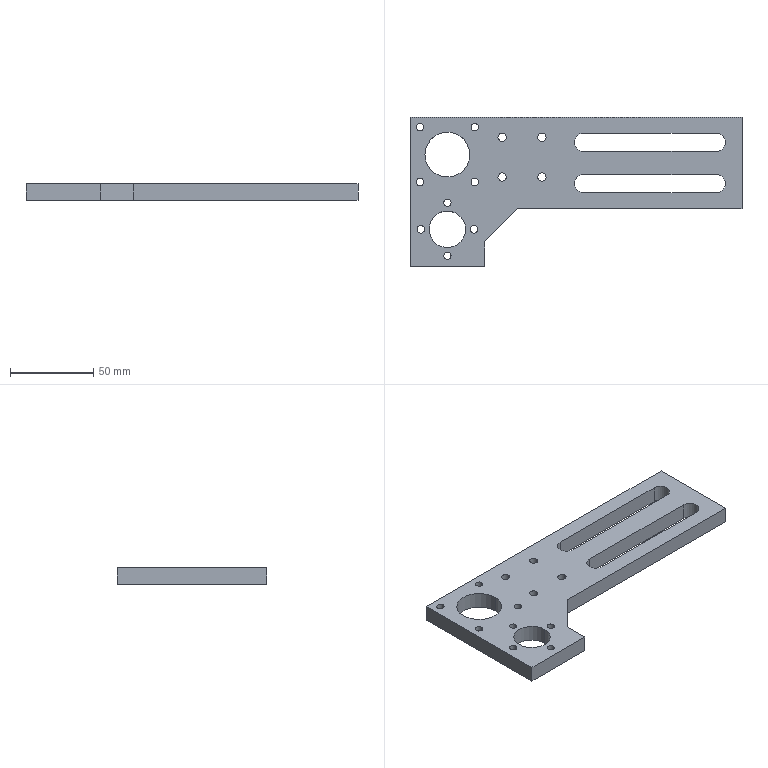Part | SolidWorks | features Chamfer 1, Extrusion 1, ICE 1 | 1 solid | 47 faces | box 200 x 90 x 10 mm | volume 96665 mm3 | cylinder 34 | plane 13 | commonest cylinder face diameters 4.5 x16 5 x8 11 x6 22 x2 27 x2